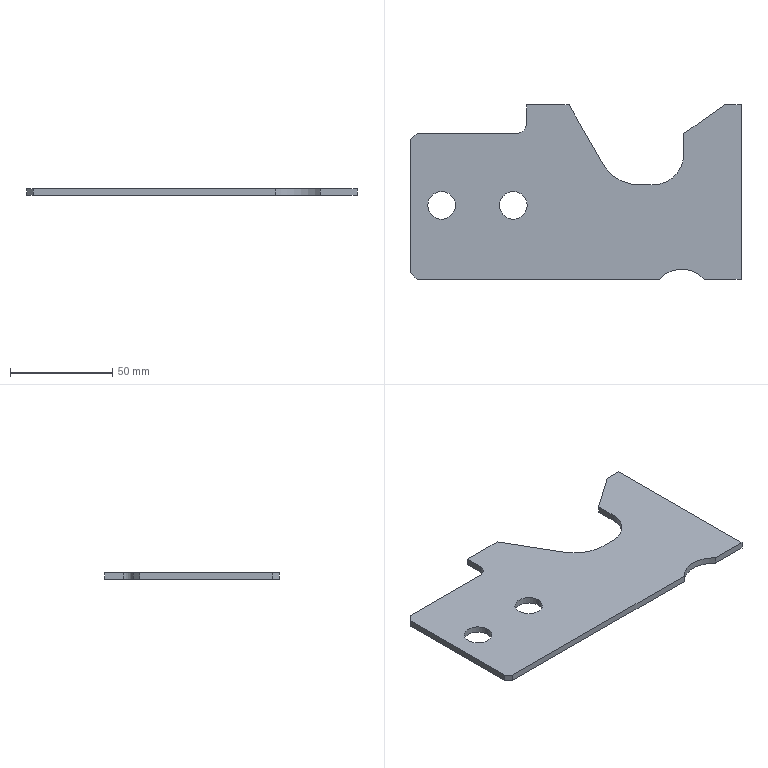Part | SolidWorks | features Fillet 3, Chamfer 1, FlatPattern 1, SMBaseFlange 1, SheetMetal 1 | 1 solid | 24 faces | box 161.2 x 85 x 3.2 mm | volume 34344 mm3 | plane 16 | cylinder 8 | commonest cylinder face diameters 13.5 x4 30 x2 10 x1 40 x1
STEP:
#1=CARTESIAN_POINT('',(-152.95,36.,3.2));
#2=VERTEX_POINT('',#1);
#3=CARTESIAN_POINT('',(-139.45,36.,3.2));
#4=VERTEX_POINT('',#3);
#5=CARTESIAN_POINT('',(-146.2,36.,3.2));
#6=DIRECTION('',(0.,0.,1.));
#7=DIRECTION('',(1.,0.,0.));
#8=AXIS2_PLACEMENT_3D('',#5,#6,#7);
#9=CIRCLE('',#8,6.75);
#10=EDGE_CURVE('',#2,#4,#9,.T.);
#11=ORIENTED_EDGE('',*,*,#10,.T.);
#12=CARTESIAN_POINT('',(-139.45,36.,0.));
#13=VERTEX_POINT('',#12);
#14=CARTESIAN_POINT('',(-139.45,36.,3.2));
#15=DIRECTION('',(0.,0.,-1.));
#16=VECTOR('',#15,1000.);
#17=LINE('',#14,#16);
#18=EDGE_CURVE('',#4,#13,#17,.T.);
#19=ORIENTED_EDGE('',*,*,#18,.T.);
#20=CARTESIAN_POINT('',(-152.95,36.,0.));
#21=VERTEX_POINT('',#20);
#22=CARTESIAN_POINT('',(-146.2,36.,0.));
#23=DIRECTION('',(0.,0.,1.));
#24=DIRECTION('',(1.,0.,0.));
#25=AXIS2_PLACEMENT_3D('',#22,#23,#24);
#26=CIRCLE('',#25,6.75);
#27=EDGE_CURVE('',#21,#13,#26,.T.);
#28=ORIENTED_EDGE('',*,*,#27,.F.);
#29=CARTESIAN_POINT('',(-152.95,36.,3.2));
#30=DIRECTION('',(0.,0.,-1.));
#31=VECTOR('',#30,1000.);
#32=LINE('',#29,#31);
#33=EDGE_CURVE('',#2,#21,#32,.T.);
#34=ORIENTED_EDGE('',*,*,#33,.F.);
#35=EDGE_LOOP('',(#11,#19,#28,#34));
#36=FACE_OUTER_BOUND('',#35,.T.);
#37=CARTESIAN_POINT('',(-146.2,36.,3.2));
#38=DIRECTION('',(0.,0.,-1.));
#39=DIRECTION('',(-1.,0.,0.));
#40=AXIS2_PLACEMENT_3D('',#37,#38,#39);
#41=CYLINDRICAL_SURFACE('',#40,6.75);
#42=ADVANCED_FACE('',(#36),#41,.F.);
#43=CARTESIAN_POINT('',(-117.95,36.,3.2));
#44=VERTEX_POINT('',#43);
#45=CARTESIAN_POINT('',(-104.45,36.,3.2));
#46=VERTEX_POINT('',#45);
#47=CARTESIAN_POINT('',(-111.2,36.,3.2));
#48=DIRECTION('',(0.,0.,1.));
#49=DIRECTION('',(1.,0.,0.));
#50=AXIS2_PLACEMENT_3D('',#47,#48,#49);
#51=CIRCLE('',#50,6.75);
#52=EDGE_CURVE('',#44,#46,#51,.T.);
#53=ORIENTED_EDGE('',*,*,#52,.T.);
#54=CARTESIAN_POINT('',(-104.45,36.,0.));
#55=VERTEX_POINT('',#54);
#56=CARTESIAN_POINT('',(-104.45,36.,3.2));
#57=DIRECTION('',(0.,0.,-1.));
#58=VECTOR('',#57,1000.);
#59=LINE('',#56,#58);
#60=EDGE_CURVE('',#46,#55,#59,.T.);
#61=ORIENTED_EDGE('',*,*,#60,.T.);
#62=CARTESIAN_POINT('',(-117.95,36.,0.));
#63=VERTEX_POINT('',#62);
#64=CARTESIAN_POINT('',(-111.2,36.,0.));
#65=DIRECTION('',(0.,0.,1.));
#66=DIRECTION('',(1.,0.,0.));
#67=AXIS2_PLACEMENT_3D('',#64,#65,#66);
#68=CIRCLE('',#67,6.75);
#69=EDGE_CURVE('',#63,#55,#68,.T.);
#70=ORIENTED_EDGE('',*,*,#69,.F.);
#71=CARTESIAN_POINT('',(-117.95,36.,3.2));
#72=DIRECTION('',(0.,0.,-1.));
#73=VECTOR('',#72,1000.);
#74=LINE('',#71,#73);
#75=EDGE_CURVE('',#44,#63,#74,.T.);
#76=ORIENTED_EDGE('',*,*,#75,.F.);
#77=EDGE_LOOP('',(#53,#61,#70,#76));
#78=FACE_OUTER_BOUND('',#77,.T.);
#79=CARTESIAN_POINT('',(-111.2,36.,3.2));
#80=DIRECTION('',(0.,0.,-1.));
#81=DIRECTION('',(-1.,0.,0.));
#82=AXIS2_PLACEMENT_3D('',#79,#80,#81);
#83=CYLINDRICAL_SURFACE('',#82,6.75);
#84=ADVANCED_FACE('',(#78),#83,.F.);
#85=ORIENTED_EDGE('',*,*,#52,.F.);
#86=CARTESIAN_POINT('',(-111.2,36.,3.2));
#87=DIRECTION('',(0.,0.,1.));
#88=DIRECTION('',(1.,0.,0.));
#89=AXIS2_PLACEMENT_3D('',#86,#87,#88);
#90=CIRCLE('',#89,6.75);
#91=EDGE_CURVE('',#46,#44,#90,.T.);
#92=ORIENTED_EDGE('',*,*,#91,.F.);
#93=EDGE_LOOP('',(#85,#92));
#94=FACE_BOUND('',#93,.T.);
#95=CARTESIAN_POINT('',(-104.7,85.,3.2));
#96=VERTEX_POINT('',#95);
#97=CARTESIAN_POINT('',(-104.7,76.,3.2));
#98=VERTEX_POINT('',#97);
#99=CARTESIAN_POINT('',(-104.7,71.,3.2));
#100=DIRECTION('',(0.,-1.,0.));
#101=VECTOR('',#100,1000.);
#102=LINE('',#99,#101);
#103=EDGE_CURVE('',#96,#98,#102,.T.);
#104=ORIENTED_EDGE('',*,*,#103,.T.);
#105=CARTESIAN_POINT('',(-109.7,71.,3.2));
#106=VERTEX_POINT('',#105);
#107=CARTESIAN_POINT('',(-109.7,76.,3.2));
#108=DIRECTION('',(0.,0.,-1.));
#109=DIRECTION('',(1.,0.,0.));
#110=AXIS2_PLACEMENT_3D('',#107,#108,#109);
#111=CIRCLE('',#110,5.);
#112=EDGE_CURVE('',#98,#106,#111,.T.);
#113=ORIENTED_EDGE('',*,*,#112,.T.);
#114=CARTESIAN_POINT('',(-158.2,71.,3.2));
#115=VERTEX_POINT('',#114);
#116=CARTESIAN_POINT('',(-161.2,71.,3.2));
#117=DIRECTION('',(-1.,0.,0.));
#118=VECTOR('',#117,1000.);
#119=LINE('',#116,#118);
#120=EDGE_CURVE('',#106,#115,#119,.T.);
#121=ORIENTED_EDGE('',*,*,#120,.T.);
#122=CARTESIAN_POINT('',(-161.2,68.,3.2));
#123=VERTEX_POINT('',#122);
#124=CARTESIAN_POINT('',(-134.201,94.999,3.2));
#125=DIRECTION('',(-0.7071,-0.7071,0.));
#126=VECTOR('',#125,1000.);
#127=LINE('',#124,#126);
#128=EDGE_CURVE('',#115,#123,#127,.T.);
#129=ORIENTED_EDGE('',*,*,#128,.T.);
#130=CARTESIAN_POINT('',(-161.2,3.,3.2));
#131=VERTEX_POINT('',#130);
#132=CARTESIAN_POINT('',(-161.2,0.,3.2));
#133=DIRECTION('',(0.,-1.,0.));
#134=VECTOR('',#133,1000.);
#135=LINE('',#132,#134);
#136=EDGE_CURVE('',#123,#131,#135,.T.);
#137=ORIENTED_EDGE('',*,*,#136,.T.);
#138=CARTESIAN_POINT('',(-158.2,0.,3.2));
#139=VERTEX_POINT('',#138);
#140=CARTESIAN_POINT('',(-88.501,-69.699,3.2));
#141=DIRECTION('',(0.7071,-0.7071,0.));
#142=VECTOR('',#141,1000.);
#143=LINE('',#140,#142);
#144=EDGE_CURVE('',#131,#139,#143,.T.);
#145=ORIENTED_EDGE('',*,*,#144,.T.);
#146=CARTESIAN_POINT('',(-40.,0.,3.2));
#147=VERTEX_POINT('',#146);
#148=CARTESIAN_POINT('',(-40.,0.,3.2));
#149=DIRECTION('',(1.,0.,0.));
#150=VECTOR('',#149,1000.);
#151=LINE('',#148,#150);
#152=EDGE_CURVE('',#139,#147,#151,.T.);
#153=ORIENTED_EDGE('',*,*,#152,.T.);
#154=CARTESIAN_POINT('',(-18.004,0.,3.2));
#155=VERTEX_POINT('',#154);
#156=CARTESIAN_POINT('',(-29.002,-10.2,3.2));
#157=DIRECTION('',(0.,0.,-1.));
#158=DIRECTION('',(1.,0.,0.));
#159=AXIS2_PLACEMENT_3D('',#156,#157,#158);
#160=CIRCLE('',#159,15.);
#161=EDGE_CURVE('',#147,#155,#160,.T.);
#162=ORIENTED_EDGE('',*,*,#161,.T.);
#163=CARTESIAN_POINT('',(0.,0.,3.2));
#164=VERTEX_POINT('',#163);
#165=CARTESIAN_POINT('',(0.,0.,3.2));
#166=DIRECTION('',(1.,0.,0.));
#167=VECTOR('',#166,1000.);
#168=LINE('',#165,#167);
#169=EDGE_CURVE('',#155,#164,#168,.T.);
#170=ORIENTED_EDGE('',*,*,#169,.T.);
#171=CARTESIAN_POINT('',(0.,85.,3.2));
#172=VERTEX_POINT('',#171);
#173=CARTESIAN_POINT('',(0.,85.,3.2));
#174=DIRECTION('',(0.,1.,0.));
#175=VECTOR('',#174,1000.);
#176=LINE('',#173,#175);
#177=EDGE_CURVE('',#164,#172,#176,.T.);
#178=ORIENTED_EDGE('',*,*,#177,.T.);
#179=CARTESIAN_POINT('',(-8.,85.,3.2));
#180=VERTEX_POINT('',#179);
#181=CARTESIAN_POINT('',(-8.,85.,3.2));
#182=DIRECTION('',(-1.,0.,0.));
#183=VECTOR('',#182,1000.);
#184=LINE('',#181,#183);
#185=EDGE_CURVE('',#172,#180,#184,.T.);
#186=ORIENTED_EDGE('',*,*,#185,.T.);
#187=CARTESIAN_POINT('',(-28.,71.,3.2));
#188=VERTEX_POINT('',#187);
#189=CARTESIAN_POINT('',(-28.,71.,3.2));
#190=DIRECTION('',(-0.8192,-0.5735,0.));
#191=VECTOR('',#190,1000.);
#192=LINE('',#189,#191);
#193=EDGE_CURVE('',#180,#188,#192,.T.);
#194=ORIENTED_EDGE('',*,*,#193,.T.);
#195=CARTESIAN_POINT('',(-28.,61.,3.2));
#196=VERTEX_POINT('',#195);
#197=CARTESIAN_POINT('',(-28.,46.,3.2));
#198=DIRECTION('',(0.,-1.,0.));
#199=VECTOR('',#198,1000.);
#200=LINE('',#197,#199);
#201=EDGE_CURVE('',#188,#196,#200,.T.);
#202=ORIENTED_EDGE('',*,*,#201,.T.);
#203=CARTESIAN_POINT('',(-43.,46.,3.2));
#204=VERTEX_POINT('',#203);
#205=CARTESIAN_POINT('',(-43.,61.,3.2));
#206=DIRECTION('',(0.,0.,-1.));
#207=DIRECTION('',(1.,0.,0.));
#208=AXIS2_PLACEMENT_3D('',#205,#206,#207);
#209=CIRCLE('',#208,15.);
#210=EDGE_CURVE('',#196,#204,#209,.T.);
#211=ORIENTED_EDGE('',*,*,#210,.T.);
#212=CARTESIAN_POINT('',(-49.949,46.,3.2));
#213=VERTEX_POINT('',#212);
#214=CARTESIAN_POINT('',(-61.5,46.,3.2));
#215=DIRECTION('',(-1.,0.,0.));
#216=VECTOR('',#215,1000.);
#217=LINE('',#214,#216);
#218=EDGE_CURVE('',#204,#213,#217,.T.);
#219=ORIENTED_EDGE('',*,*,#218,.T.);
#220=CARTESIAN_POINT('',(-67.272,56.006,3.2));
#221=VERTEX_POINT('',#220);
#222=CARTESIAN_POINT('',(-49.949,66.,3.2));
#223=DIRECTION('',(0.,0.,-1.));
#224=DIRECTION('',(1.,0.,0.));
#225=AXIS2_PLACEMENT_3D('',#222,#223,#224);
#226=CIRCLE('',#225,20.);
#227=EDGE_CURVE('',#213,#221,#226,.T.);
#228=ORIENTED_EDGE('',*,*,#227,.T.);
#229=CARTESIAN_POINT('',(-84.,85.,3.2));
#230=VERTEX_POINT('',#229);
#231=CARTESIAN_POINT('',(-84.,85.,3.2));
#232=DIRECTION('',(-0.4997,0.8662,0.));
#233=VECTOR('',#232,1000.);
#234=LINE('',#231,#233);
#235=EDGE_CURVE('',#221,#230,#234,.T.);
#236=ORIENTED_EDGE('',*,*,#235,.T.);
#237=CARTESIAN_POINT('',(-104.7,85.,3.2));
#238=DIRECTION('',(-1.,0.,0.));
#239=VECTOR('',#238,1000.);
#240=LINE('',#237,#239);
#241=EDGE_CURVE('',#230,#96,#240,.T.);
#242=ORIENTED_EDGE('',*,*,#241,.T.);
#243=EDGE_LOOP('',(#104,#113,#121,#129,#137,#145,#153,#162,#170,#178,#186,#194,#202,#211,#219,#228,#236,#242));
#244=FACE_OUTER_BOUND('',#243,.T.);
#245=ORIENTED_EDGE('',*,*,#10,.F.);
#246=CARTESIAN_POINT('',(-146.2,36.,3.2));
#247=DIRECTION('',(0.,0.,1.));
#248=DIRECTION('',(1.,0.,0.));
#249=AXIS2_PLACEMENT_3D('',#246,#247,#248);
#250=CIRCLE('',#249,6.75);
#251=EDGE_CURVE('',#4,#2,#250,.T.);
#252=ORIENTED_EDGE('',*,*,#251,.F.);
#253=EDGE_LOOP('',(#245,#252));
#254=FACE_BOUND('',#253,.T.);
#255=CARTESIAN_POINT('',(-29.002,-10.2,3.2));
#256=DIRECTION('',(0.,0.,1.));
#257=DIRECTION('',(1.,0.,0.));
#258=AXIS2_PLACEMENT_3D('',#255,#256,#257);
#259=PLANE('',#258);
#260=ADVANCED_FACE('',(#94,#244,#254),#259,.T.);
#261=CARTESIAN_POINT('',(-161.2,68.,0.));
#262=VERTEX_POINT('',#261);
#263=CARTESIAN_POINT('',(-161.2,3.,0.));
#264=VERTEX_POINT('',#263);
#265=CARTESIAN_POINT('',(-161.2,0.,0.));
#266=DIRECTION('',(0.,-1.,0.));
#267=VECTOR('',#266,1000.);
#268=LINE('',#265,#267);
#269=EDGE_CURVE('',#262,#264,#268,.T.);
#270=ORIENTED_EDGE('',*,*,#269,.F.);
#271=CARTESIAN_POINT('',(-158.2,71.,0.));
#272=VERTEX_POINT('',#271);
#273=CARTESIAN_POINT('',(-161.2,68.,0.));
#274=DIRECTION('',(0.7071,0.7071,0.));
#275=VECTOR('',#274,1000.);
#276=LINE('',#273,#275);
#277=EDGE_CURVE('',#262,#272,#276,.T.);
#278=ORIENTED_EDGE('',*,*,#277,.T.);
#279=CARTESIAN_POINT('',(-109.7,71.,0.));
#280=VERTEX_POINT('',#279);
#281=CARTESIAN_POINT('',(-161.2,71.,0.));
#282=DIRECTION('',(-1.,0.,0.));
#283=VECTOR('',#282,1000.);
#284=LINE('',#281,#283);
#285=EDGE_CURVE('',#280,#272,#284,.T.);
#286=ORIENTED_EDGE('',*,*,#285,.F.);
#287=CARTESIAN_POINT('',(-104.7,76.,0.));
#288=VERTEX_POINT('',#287);
#289=CARTESIAN_POINT('',(-109.7,76.,0.));
#290=DIRECTION('',(0.,0.,1.));
#291=DIRECTION('',(1.,0.,0.));
#292=AXIS2_PLACEMENT_3D('',#289,#290,#291);
#293=CIRCLE('',#292,5.);
#294=EDGE_CURVE('',#280,#288,#293,.T.);
#295=ORIENTED_EDGE('',*,*,#294,.T.);
#296=CARTESIAN_POINT('',(-104.7,85.,0.));
#297=VERTEX_POINT('',#296);
#298=CARTESIAN_POINT('',(-104.7,71.,0.));
#299=DIRECTION('',(0.,-1.,0.));
#300=VECTOR('',#299,1000.);
#301=LINE('',#298,#300);
#302=EDGE_CURVE('',#297,#288,#301,.T.);
#303=ORIENTED_EDGE('',*,*,#302,.F.);
#304=CARTESIAN_POINT('',(-84.,85.,0.));
#305=VERTEX_POINT('',#304);
#306=CARTESIAN_POINT('',(-104.7,85.,0.));
#307=DIRECTION('',(-1.,0.,0.));
#308=VECTOR('',#307,1000.);
#309=LINE('',#306,#308);
#310=EDGE_CURVE('',#305,#297,#309,.T.);
#311=ORIENTED_EDGE('',*,*,#310,.F.);
#312=CARTESIAN_POINT('',(-67.272,56.006,0.));
#313=VERTEX_POINT('',#312);
#314=CARTESIAN_POINT('',(-84.,85.,0.));
#315=DIRECTION('',(-0.4997,0.8662,0.));
#316=VECTOR('',#315,1000.);
#317=LINE('',#314,#316);
#318=EDGE_CURVE('',#313,#305,#317,.T.);
#319=ORIENTED_EDGE('',*,*,#318,.F.);
#320=CARTESIAN_POINT('',(-49.949,46.,0.));
#321=VERTEX_POINT('',#320);
#322=CARTESIAN_POINT('',(-49.949,66.,0.));
#323=DIRECTION('',(0.,0.,1.));
#324=DIRECTION('',(1.,0.,0.));
#325=AXIS2_PLACEMENT_3D('',#322,#323,#324);
#326=CIRCLE('',#325,20.);
#327=EDGE_CURVE('',#313,#321,#326,.T.);
#328=ORIENTED_EDGE('',*,*,#327,.T.);
#329=CARTESIAN_POINT('',(-43.,46.,0.));
#330=VERTEX_POINT('',#329);
#331=CARTESIAN_POINT('',(-61.5,46.,0.));
#332=DIRECTION('',(-1.,0.,0.));
#333=VECTOR('',#332,1000.);
#334=LINE('',#331,#333);
#335=EDGE_CURVE('',#330,#321,#334,.T.);
#336=ORIENTED_EDGE('',*,*,#335,.F.);
#337=CARTESIAN_POINT('',(-28.,61.,0.));
#338=VERTEX_POINT('',#337);
#339=CARTESIAN_POINT('',(-43.,61.,0.));
#340=DIRECTION('',(0.,0.,1.));
#341=DIRECTION('',(1.,0.,0.));
#342=AXIS2_PLACEMENT_3D('',#339,#340,#341);
#343=CIRCLE('',#342,15.);
#344=EDGE_CURVE('',#330,#338,#343,.T.);
#345=ORIENTED_EDGE('',*,*,#344,.T.);
#346=CARTESIAN_POINT('',(-28.,71.,0.));
#347=VERTEX_POINT('',#346);
#348=CARTESIAN_POINT('',(-28.,46.,0.));
#349=DIRECTION('',(0.,-1.,0.));
#350=VECTOR('',#349,1000.);
#351=LINE('',#348,#350);
#352=EDGE_CURVE('',#347,#338,#351,.T.);
#353=ORIENTED_EDGE('',*,*,#352,.F.);
#354=CARTESIAN_POINT('',(-8.,85.,0.));
#355=VERTEX_POINT('',#354);
#356=CARTESIAN_POINT('',(-28.,71.,0.));
#357=DIRECTION('',(-0.8192,-0.5735,0.));
#358=VECTOR('',#357,1000.);
#359=LINE('',#356,#358);
#360=EDGE_CURVE('',#355,#347,#359,.T.);
#361=ORIENTED_EDGE('',*,*,#360,.F.);
#362=CARTESIAN_POINT('',(0.,85.,0.));
#363=VERTEX_POINT('',#362);
#364=CARTESIAN_POINT('',(-8.,85.,0.));
#365=DIRECTION('',(-1.,0.,0.));
#366=VECTOR('',#365,1000.);
#367=LINE('',#364,#366);
#368=EDGE_CURVE('',#363,#355,#367,.T.);
#369=ORIENTED_EDGE('',*,*,#368,.F.);
#370=CARTESIAN_POINT('',(0.,0.,0.));
#371=VERTEX_POINT('',#370);
#372=CARTESIAN_POINT('',(0.,85.,0.));
#373=DIRECTION('',(0.,1.,0.));
#374=VECTOR('',#373,1000.);
#375=LINE('',#372,#374);
#376=EDGE_CURVE('',#371,#363,#375,.T.);
#377=ORIENTED_EDGE('',*,*,#376,.F.);
#378=CARTESIAN_POINT('',(-18.004,0.,0.));
#379=VERTEX_POINT('',#378);
#380=CARTESIAN_POINT('',(0.,0.,0.));
#381=DIRECTION('',(1.,0.,0.));
#382=VECTOR('',#381,1000.);
#383=LINE('',#380,#382);
#384=EDGE_CURVE('',#379,#371,#383,.T.);
#385=ORIENTED_EDGE('',*,*,#384,.F.);
#386=CARTESIAN_POINT('',(-40.,0.,0.));
#387=VERTEX_POINT('',#386);
#388=CARTESIAN_POINT('',(-29.002,-10.2,0.));
#389=DIRECTION('',(0.,0.,-1.));
#390=DIRECTION('',(1.,0.,0.));
#391=AXIS2_PLACEMENT_3D('',#388,#389,#390);
#392=CIRCLE('',#391,15.);
#393=EDGE_CURVE('',#387,#379,#392,.T.);
#394=ORIENTED_EDGE('',*,*,#393,.F.);
#395=CARTESIAN_POINT('',(-158.2,0.,0.));
#396=VERTEX_POINT('',#395);
#397=CARTESIAN_POINT('',(-40.,0.,0.));
#398=DIRECTION('',(1.,0.,0.));
#399=VECTOR('',#398,1000.);
#400=LINE('',#397,#399);
#401=EDGE_CURVE('',#396,#387,#400,.T.);
#402=ORIENTED_EDGE('',*,*,#401,.F.);
#403=CARTESIAN_POINT('',(-158.2,0.,0.));
#404=DIRECTION('',(-0.7071,0.7071,0.));
#405=VECTOR('',#404,1000.);
#406=LINE('',#403,#405);
#407=EDGE_CURVE('',#396,#264,#406,.T.);
#408=ORIENTED_EDGE('',*,*,#407,.T.);
#409=EDGE_LOOP('',(#270,#278,#286,#295,#303,#311,#319,#328,#336,#345,#353,#361,#369,#377,#385,#394,#402,#408));
#410=FACE_OUTER_BOUND('',#409,.T.);
#411=ORIENTED_EDGE('',*,*,#69,.T.);
#412=CARTESIAN_POINT('',(-111.2,36.,0.));
#413=DIRECTION('',(0.,0.,1.));
#414=DIRECTION('',(1.,0.,0.));
#415=AXIS2_PLACEMENT_3D('',#412,#413,#414);
#416=CIRCLE('',#415,6.75);
#417=EDGE_CURVE('',#55,#63,#416,.T.);
#418=ORIENTED_EDGE('',*,*,#417,.T.);
#419=EDGE_LOOP('',(#411,#418));
#420=FACE_BOUND('',#419,.T.);
#421=ORIENTED_EDGE('',*,*,#27,.T.);
#422=CARTESIAN_POINT('',(-146.2,36.,0.));
#423=DIRECTION('',(0.,0.,1.));
#424=DIRECTION('',(1.,0.,0.));
#425=AXIS2_PLACEMENT_3D('',#422,#423,#424);
#426=CIRCLE('',#425,6.75);
#427=EDGE_CURVE('',#13,#21,#426,.T.);
#428=ORIENTED_EDGE('',*,*,#427,.T.);
#429=EDGE_LOOP('',(#421,#428));
#430=FACE_BOUND('',#429,.T.);
#431=CARTESIAN_POINT('',(-29.002,-10.2,0.));
#432=DIRECTION('',(0.,0.,1.));
#433=DIRECTION('',(1.,0.,0.));
#434=AXIS2_PLACEMENT_3D('',#431,#432,#433);
#435=PLANE('',#434);
#436=ADVANCED_FACE('',(#410,#420,#430),#435,.F.);
#437=ORIENTED_EDGE('',*,*,#376,.T.);
#438=CARTESIAN_POINT('',(0.,85.,3.2));
#439=DIRECTION('',(0.,0.,-1.));
#440=VECTOR('',#439,1000.);
#441=LINE('',#438,#440);
#442=EDGE_CURVE('',#172,#363,#441,.T.);
#443=ORIENTED_EDGE('',*,*,#442,.F.);
#444=ORIENTED_EDGE('',*,*,#177,.F.);
#445=CARTESIAN_POINT('',(0.,0.,3.2));
#446=DIRECTION('',(0.,0.,-1.));
#447=VECTOR('',#446,1000.);
#448=LINE('',#445,#447);
#449=EDGE_CURVE('',#164,#371,#448,.T.);
#450=ORIENTED_EDGE('',*,*,#449,.T.);
#451=EDGE_LOOP('',(#437,#443,#444,#450));
#452=FACE_OUTER_BOUND('',#451,.T.);
#453=CARTESIAN_POINT('',(0.,85.,3.2));
#454=DIRECTION('',(-1.,0.,0.));
#455=DIRECTION('',(0.,0.,1.));
#456=AXIS2_PLACEMENT_3D('',#453,#454,#455);
#457=PLANE('',#456);
#458=ADVANCED_FACE('',(#452),#457,.F.);
#459=ORIENTED_EDGE('',*,*,#368,.T.);
#460=CARTESIAN_POINT('',(-8.,85.,3.2));
#461=DIRECTION('',(0.,0.,-1.));
#462=VECTOR('',#461,1000.);
#463=LINE('',#460,#462);
#464=EDGE_CURVE('',#180,#355,#463,.T.);
#465=ORIENTED_EDGE('',*,*,#464,.F.);
#466=ORIENTED_EDGE('',*,*,#185,.F.);
#467=ORIENTED_EDGE('',*,*,#442,.T.);
#468=EDGE_LOOP('',(#459,#465,#466,#467));
#469=FACE_OUTER_BOUND('',#468,.T.);
#470=CARTESIAN_POINT('',(-8.,85.,3.2));
#471=DIRECTION('',(0.,-1.,0.));
#472=DIRECTION('',(0.,0.,-1.));
#473=AXIS2_PLACEMENT_3D('',#470,#471,#472);
#474=PLANE('',#473);
#475=ADVANCED_FACE('',(#469),#474,.F.);
#476=ORIENTED_EDGE('',*,*,#360,.T.);
#477=CARTESIAN_POINT('',(-28.,71.,3.2));
#478=DIRECTION('',(0.,0.,-1.));
#479=VECTOR('',#478,1000.);
#480=LINE('',#477,#479);
#481=EDGE_CURVE('',#188,#347,#480,.T.);
#482=ORIENTED_EDGE('',*,*,#481,.F.);
#483=ORIENTED_EDGE('',*,*,#193,.F.);
#484=ORIENTED_EDGE('',*,*,#464,.T.);
#485=EDGE_LOOP('',(#476,#482,#483,#484));
#486=FACE_OUTER_BOUND('',#485,.T.);
#487=CARTESIAN_POINT('',(-28.,71.,3.2));
#488=DIRECTION('',(0.5735,-0.8192,0.));
#489=DIRECTION('',(0.8192,0.5735,0.));
#490=AXIS2_PLACEMENT_3D('',#487,#488,#489);
#491=PLANE('',#490);
#492=ADVANCED_FACE('',(#486),#491,.F.);
#493=ORIENTED_EDGE('',*,*,#352,.T.);
#494=CARTESIAN_POINT('',(-28.,61.,3.2));
#495=DIRECTION('',(0.,0.,1.));
#496=VECTOR('',#495,1000.);
#497=LINE('',#494,#496);
#498=EDGE_CURVE('',#338,#196,#497,.T.);
#499=ORIENTED_EDGE('',*,*,#498,.T.);
#500=ORIENTED_EDGE('',*,*,#201,.F.);
#501=ORIENTED_EDGE('',*,*,#481,.T.);
#502=EDGE_LOOP('',(#493,#499,#500,#501));
#503=FACE_OUTER_BOUND('',#502,.T.);
#504=CARTESIAN_POINT('',(-28.,46.,3.2));
#505=DIRECTION('',(1.,0.,0.));
#506=DIRECTION('',(0.,0.,-1.));
#507=AXIS2_PLACEMENT_3D('',#504,#505,#506);
#508=PLANE('',#507);
#509=ADVANCED_FACE('',(#503),#508,.F.);
#510=ORIENTED_EDGE('',*,*,#218,.F.);
#511=CARTESIAN_POINT('',(-43.,46.,0.));
#512=DIRECTION('',(0.,0.,-1.));
#513=VECTOR('',#512,1000.);
#514=LINE('',#511,#513);
#515=EDGE_CURVE('',#204,#330,#514,.T.);
#516=ORIENTED_EDGE('',*,*,#515,.T.);
#517=ORIENTED_EDGE('',*,*,#335,.T.);
#518=CARTESIAN_POINT('',(-49.949,46.,3.2));
#519=DIRECTION('',(0.,0.,1.));
#520=VECTOR('',#519,1000.);
#521=LINE('',#518,#520);
#522=EDGE_CURVE('',#321,#213,#521,.T.);
#523=ORIENTED_EDGE('',*,*,#522,.T.);
#524=EDGE_LOOP('',(#510,#516,#517,#523));
#525=FACE_OUTER_BOUND('',#524,.T.);
#526=CARTESIAN_POINT('',(-61.5,46.,3.2));
#527=DIRECTION('',(0.,-1.,0.));
#528=DIRECTION('',(0.,0.,-1.));
#529=AXIS2_PLACEMENT_3D('',#526,#527,#528);
#530=PLANE('',#529);
#531=ADVANCED_FACE('',(#525),#530,.F.);
#532=ORIENTED_EDGE('',*,*,#235,.F.);
#533=CARTESIAN_POINT('',(-67.272,56.006,0.));
#534=DIRECTION('',(0.,0.,-1.));
#535=VECTOR('',#534,1000.);
#536=LINE('',#533,#535);
#537=EDGE_CURVE('',#221,#313,#536,.T.);
#538=ORIENTED_EDGE('',*,*,#537,.T.);
#539=ORIENTED_EDGE('',*,*,#318,.T.);
#540=CARTESIAN_POINT('',(-84.,85.,3.2));
#541=DIRECTION('',(0.,0.,-1.));
#542=VECTOR('',#541,1000.);
#543=LINE('',#540,#542);
#544=EDGE_CURVE('',#230,#305,#543,.T.);
#545=ORIENTED_EDGE('',*,*,#544,.F.);
#546=EDGE_LOOP('',(#532,#538,#539,#545));
#547=FACE_OUTER_BOUND('',#546,.T.);
#548=CARTESIAN_POINT('',(-84.,85.,3.2));
#549=DIRECTION('',(-0.8662,-0.4997,0.));
#550=DIRECTION('',(0.4997,-0.8662,0.));
#551=AXIS2_PLACEMENT_3D('',#548,#549,#550);
#552=PLANE('',#551);
#553=ADVANCED_FACE('',(#547),#552,.F.);
#554=ORIENTED_EDGE('',*,*,#310,.T.);
#555=CARTESIAN_POINT('',(-104.7,85.,3.2));
#556=DIRECTION('',(0.,0.,-1.));
#557=VECTOR('',#556,1000.);
#558=LINE('',#555,#557);
#559=EDGE_CURVE('',#96,#297,#558,.T.);
#560=ORIENTED_EDGE('',*,*,#559,.F.);
#561=ORIENTED_EDGE('',*,*,#241,.F.);
#562=ORIENTED_EDGE('',*,*,#544,.T.);
#563=EDGE_LOOP('',(#554,#560,#561,#562));
#564=FACE_OUTER_BOUND('',#563,.T.);
#565=CARTESIAN_POINT('',(-104.7,85.,3.2));
#566=DIRECTION('',(0.,-1.,0.));
#567=DIRECTION('',(0.,0.,-1.));
#568=AXIS2_PLACEMENT_3D('',#565,#566,#567);
#569=PLANE('',#568);
#570=ADVANCED_FACE('',(#564),#569,.F.);
#571=ORIENTED_EDGE('',*,*,#302,.T.);
#572=CARTESIAN_POINT('',(-104.7,76.,3.2));
#573=DIRECTION('',(0.,0.,1.));
#574=VECTOR('',#573,1000.);
#575=LINE('',#572,#574);
#576=EDGE_CURVE('',#288,#98,#575,.T.);
#577=ORIENTED_EDGE('',*,*,#576,.T.);
#578=ORIENTED_EDGE('',*,*,#103,.F.);
#579=ORIENTED_EDGE('',*,*,#559,.T.);
#580=EDGE_LOOP('',(#571,#577,#578,#579));
#581=FACE_OUTER_BOUND('',#580,.T.);
#582=CARTESIAN_POINT('',(-104.7,71.,3.2));
#583=DIRECTION('',(1.,0.,0.));
#584=DIRECTION('',(0.,0.,-1.));
#585=AXIS2_PLACEMENT_3D('',#582,#583,#584);
#586=PLANE('',#585);
#587=ADVANCED_FACE('',(#581),#586,.F.);
#588=ORIENTED_EDGE('',*,*,#120,.F.);
#589=CARTESIAN_POINT('',(-109.7,71.,0.));
#590=DIRECTION('',(0.,0.,-1.));
#591=VECTOR('',#590,1000.);
#592=LINE('',#589,#591);
#593=EDGE_CURVE('',#106,#280,#592,.T.);
#594=ORIENTED_EDGE('',*,*,#593,.T.);
#595=ORIENTED_EDGE('',*,*,#285,.T.);
#596=CARTESIAN_POINT('',(-158.2,71.,3.2));
#597=DIRECTION('',(0.,0.,1.));
#598=VECTOR('',#597,1000.);
#599=LINE('',#596,#598);
#600=EDGE_CURVE('',#272,#115,#599,.T.);
#601=ORIENTED_EDGE('',*,*,#600,.T.);
#602=EDGE_LOOP('',(#588,#594,#595,#601));
#603=FACE_OUTER_BOUND('',#602,.T.);
#604=CARTESIAN_POINT('',(-161.2,71.,3.2));
#605=DIRECTION('',(0.,-1.,0.));
#606=DIRECTION('',(0.,0.,-1.));
#607=AXIS2_PLACEMENT_3D('',#604,#605,#606);
#608=PLANE('',#607);
#609=ADVANCED_FACE('',(#603),#608,.F.);
#610=ORIENTED_EDGE('',*,*,#136,.F.);
#611=CARTESIAN_POINT('',(-161.2,68.,3.2));
#612=DIRECTION('',(0.,0.,-1.));
#613=VECTOR('',#612,1000.);
#614=LINE('',#611,#613);
#615=EDGE_CURVE('',#123,#262,#614,.T.);
#616=ORIENTED_EDGE('',*,*,#615,.T.);
#617=ORIENTED_EDGE('',*,*,#269,.T.);
#618=CARTESIAN_POINT('',(-161.2,3.,3.2));
#619=DIRECTION('',(0.,0.,1.));
#620=VECTOR('',#619,1000.);
#621=LINE('',#618,#620);
#622=EDGE_CURVE('',#264,#131,#621,.T.);
#623=ORIENTED_EDGE('',*,*,#622,.T.);
#624=EDGE_LOOP('',(#610,#616,#617,#623));
#625=FACE_OUTER_BOUND('',#624,.T.);
#626=CARTESIAN_POINT('',(-161.2,0.,3.2));
#627=DIRECTION('',(1.,0.,0.));
#628=DIRECTION('',(0.,0.,-1.));
#629=AXIS2_PLACEMENT_3D('',#626,#627,#628);
#630=PLANE('',#629);
#631=ADVANCED_FACE('',(#625),#630,.F.);
#632=ORIENTED_EDGE('',*,*,#152,.F.);
#633=CARTESIAN_POINT('',(-158.2,0.,3.2));
#634=DIRECTION('',(0.,0.,-1.));
#635=VECTOR('',#634,1000.);
#636=LINE('',#633,#635);
#637=EDGE_CURVE('',#139,#396,#636,.T.);
#638=ORIENTED_EDGE('',*,*,#637,.T.);
#639=ORIENTED_EDGE('',*,*,#401,.T.);
#640=CARTESIAN_POINT('',(-40.,0.,3.2));
#641=DIRECTION('',(0.,0.,-1.));
#642=VECTOR('',#641,1000.);
#643=LINE('',#640,#642);
#644=EDGE_CURVE('',#147,#387,#643,.T.);
#645=ORIENTED_EDGE('',*,*,#644,.F.);
#646=EDGE_LOOP('',(#632,#638,#639,#645));
#647=FACE_OUTER_BOUND('',#646,.T.);
#648=CARTESIAN_POINT('',(-40.,0.,3.2));
#649=DIRECTION('',(0.,1.,0.));
#650=DIRECTION('',(-1.,0.,0.));
#651=AXIS2_PLACEMENT_3D('',#648,#649,#650);
#652=PLANE('',#651);
#653=ADVANCED_FACE('',(#647),#652,.F.);
#654=ORIENTED_EDGE('',*,*,#393,.T.);
#655=CARTESIAN_POINT('',(-18.004,0.,3.2));
#656=DIRECTION('',(0.,0.,-1.));
#657=VECTOR('',#656,1000.);
#658=LINE('',#655,#657);
#659=EDGE_CURVE('',#155,#379,#658,.T.);
#660=ORIENTED_EDGE('',*,*,#659,.F.);
#661=ORIENTED_EDGE('',*,*,#161,.F.);
#662=ORIENTED_EDGE('',*,*,#644,.T.);
#663=EDGE_LOOP('',(#654,#660,#661,#662));
#664=FACE_OUTER_BOUND('',#663,.T.);
#665=CARTESIAN_POINT('',(-29.002,-10.2,3.2));
#666=DIRECTION('',(0.,0.,-1.));
#667=DIRECTION('',(-1.,0.,0.));
#668=AXIS2_PLACEMENT_3D('',#665,#666,#667);
#669=CYLINDRICAL_SURFACE('',#668,15.);
#670=ADVANCED_FACE('',(#664),#669,.F.);
#671=ORIENTED_EDGE('',*,*,#384,.T.);
#672=ORIENTED_EDGE('',*,*,#449,.F.);
#673=ORIENTED_EDGE('',*,*,#169,.F.);
#674=ORIENTED_EDGE('',*,*,#659,.T.);
#675=EDGE_LOOP('',(#671,#672,#673,#674));
#676=FACE_OUTER_BOUND('',#675,.T.);
#677=CARTESIAN_POINT('',(0.,0.,3.2));
#678=DIRECTION('',(0.,1.,0.));
#679=DIRECTION('',(-1.,0.,0.));
#680=AXIS2_PLACEMENT_3D('',#677,#678,#679);
#681=PLANE('',#680);
#682=ADVANCED_FACE('',(#676),#681,.F.);
#683=ORIENTED_EDGE('',*,*,#60,.F.);
#684=ORIENTED_EDGE('',*,*,#91,.T.);
#685=ORIENTED_EDGE('',*,*,#75,.T.);
#686=ORIENTED_EDGE('',*,*,#417,.F.);
#687=EDGE_LOOP('',(#683,#684,#685,#686));
#688=FACE_OUTER_BOUND('',#687,.T.);
#689=CARTESIAN_POINT('',(-111.2,36.,3.2));
#690=DIRECTION('',(0.,0.,-1.));
#691=DIRECTION('',(-1.,0.,0.));
#692=AXIS2_PLACEMENT_3D('',#689,#690,#691);
#693=CYLINDRICAL_SURFACE('',#692,6.75);
#694=ADVANCED_FACE('',(#688),#693,.F.);
#695=ORIENTED_EDGE('',*,*,#18,.F.);
#696=ORIENTED_EDGE('',*,*,#251,.T.);
#697=ORIENTED_EDGE('',*,*,#33,.T.);
#698=ORIENTED_EDGE('',*,*,#427,.F.);
#699=EDGE_LOOP('',(#695,#696,#697,#698));
#700=FACE_OUTER_BOUND('',#699,.T.);
#701=CARTESIAN_POINT('',(-146.2,36.,3.2));
#702=DIRECTION('',(0.,0.,-1.));
#703=DIRECTION('',(-1.,0.,0.));
#704=AXIS2_PLACEMENT_3D('',#701,#702,#703);
#705=CYLINDRICAL_SURFACE('',#704,6.75);
#706=ADVANCED_FACE('',(#700),#705,.F.);
#707=ORIENTED_EDGE('',*,*,#128,.F.);
#708=ORIENTED_EDGE('',*,*,#600,.F.);
#709=ORIENTED_EDGE('',*,*,#277,.F.);
#710=ORIENTED_EDGE('',*,*,#615,.F.);
#711=EDGE_LOOP('',(#707,#708,#709,#710));
#712=FACE_OUTER_BOUND('',#711,.T.);
#713=CARTESIAN_POINT('',(-161.2,68.,3.2));
#714=DIRECTION('',(0.7071,-0.7071,0.));
#715=DIRECTION('',(0.,0.,-1.));
#716=AXIS2_PLACEMENT_3D('',#713,#714,#715);
#717=PLANE('',#716);
#718=ADVANCED_FACE('',(#712),#717,.F.);
#719=ORIENTED_EDGE('',*,*,#144,.F.);
#720=ORIENTED_EDGE('',*,*,#622,.F.);
#721=ORIENTED_EDGE('',*,*,#407,.F.);
#722=ORIENTED_EDGE('',*,*,#637,.F.);
#723=EDGE_LOOP('',(#719,#720,#721,#722));
#724=FACE_OUTER_BOUND('',#723,.T.);
#725=CARTESIAN_POINT('',(-158.2,0.,3.2));
#726=DIRECTION('',(0.7071,0.7071,0.));
#727=DIRECTION('',(0.,0.,-1.));
#728=AXIS2_PLACEMENT_3D('',#725,#726,#727);
#729=PLANE('',#728);
#730=ADVANCED_FACE('',(#724),#729,.F.);
#731=ORIENTED_EDGE('',*,*,#227,.F.);
#732=ORIENTED_EDGE('',*,*,#522,.F.);
#733=ORIENTED_EDGE('',*,*,#327,.F.);
#734=ORIENTED_EDGE('',*,*,#537,.F.);
#735=EDGE_LOOP('',(#731,#732,#733,#734));
#736=FACE_OUTER_BOUND('',#735,.T.);
#737=CARTESIAN_POINT('',(-49.949,66.,3.2));
#738=DIRECTION('',(0.,0.,1.));
#739=DIRECTION('',(1.,0.,0.));
#740=AXIS2_PLACEMENT_3D('',#737,#738,#739);
#741=CYLINDRICAL_SURFACE('',#740,20.);
#742=ADVANCED_FACE('',(#736),#741,.F.);
#743=ORIENTED_EDGE('',*,*,#210,.F.);
#744=ORIENTED_EDGE('',*,*,#498,.F.);
#745=ORIENTED_EDGE('',*,*,#344,.F.);
#746=ORIENTED_EDGE('',*,*,#515,.F.);
#747=EDGE_LOOP('',(#743,#744,#745,#746));
#748=FACE_OUTER_BOUND('',#747,.T.);
#749=CARTESIAN_POINT('',(-43.,61.,3.2));
#750=DIRECTION('',(0.,0.,1.));
#751=DIRECTION('',(1.,0.,0.));
#752=AXIS2_PLACEMENT_3D('',#749,#750,#751);
#753=CYLINDRICAL_SURFACE('',#752,15.);
#754=ADVANCED_FACE('',(#748),#753,.F.);
#755=ORIENTED_EDGE('',*,*,#112,.F.);
#756=ORIENTED_EDGE('',*,*,#576,.F.);
#757=ORIENTED_EDGE('',*,*,#294,.F.);
#758=ORIENTED_EDGE('',*,*,#593,.F.);
#759=EDGE_LOOP('',(#755,#756,#757,#758));
#760=FACE_OUTER_BOUND('',#759,.T.);
#761=CARTESIAN_POINT('',(-109.7,76.,3.2));
#762=DIRECTION('',(0.,0.,1.));
#763=DIRECTION('',(1.,0.,0.));
#764=AXIS2_PLACEMENT_3D('',#761,#762,#763);
#765=CYLINDRICAL_SURFACE('',#764,5.);
#766=ADVANCED_FACE('',(#760),#765,.F.);
#767=CLOSED_SHELL('',(#42,#84,#260,#436,#458,#475,#492,#509,#531,#553,#570,#587,#609,#631,#653,#670,#682,#694,#706,#718,#730,#742,#754,#766));
#768=MANIFOLD_SOLID_BREP('',#767);
#769=CARTESIAN_POINT('',(0.,0.,0.));
#770=DIRECTION('',(0.,0.,1.));
#771=DIRECTION('',(1.,0.,0.));
#772=AXIS2_PLACEMENT_3D('',#769,#770,#771);
#773=(LENGTH_UNIT()NAMED_UNIT(*)SI_UNIT(.MILLI.,.METRE.));
#774=UNCERTAINTY_MEASURE_WITH_UNIT(LENGTH_MEASURE(0.00001),#773,'','');
#775=(NAMED_UNIT(*)PLANE_ANGLE_UNIT()SI_UNIT($,.RADIAN.));
#776=(NAMED_UNIT(*)SI_UNIT($,.STERADIAN.)SOLID_ANGLE_UNIT());
#777=(GEOMETRIC_REPRESENTATION_CONTEXT(3)GLOBAL_UNCERTAINTY_ASSIGNED_CONTEXT((#774))GLOBAL_UNIT_ASSIGNED_CONTEXT((#773,#775,#776))REPRESENTATION_CONTEXT('',''));
#778=ADVANCED_BREP_SHAPE_REPRESENTATION('',(#768,#772),#777);